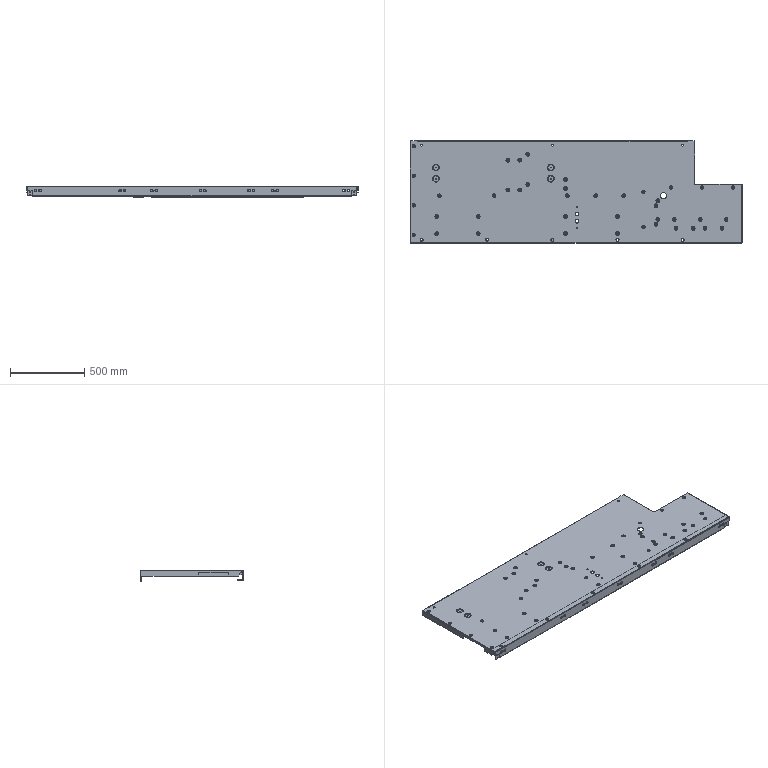Part | STEP file | 1 solid | 1194 faces | box 2240 x 691 x 80 mm | volume 4221901 mm3 | cylinder 435 | plane 393 | torus 360 | spline 6 | commonest cylinder face diameters 4.7 x66 20 x64 24 x64 20.5 x48 18 x38 5.3 x30